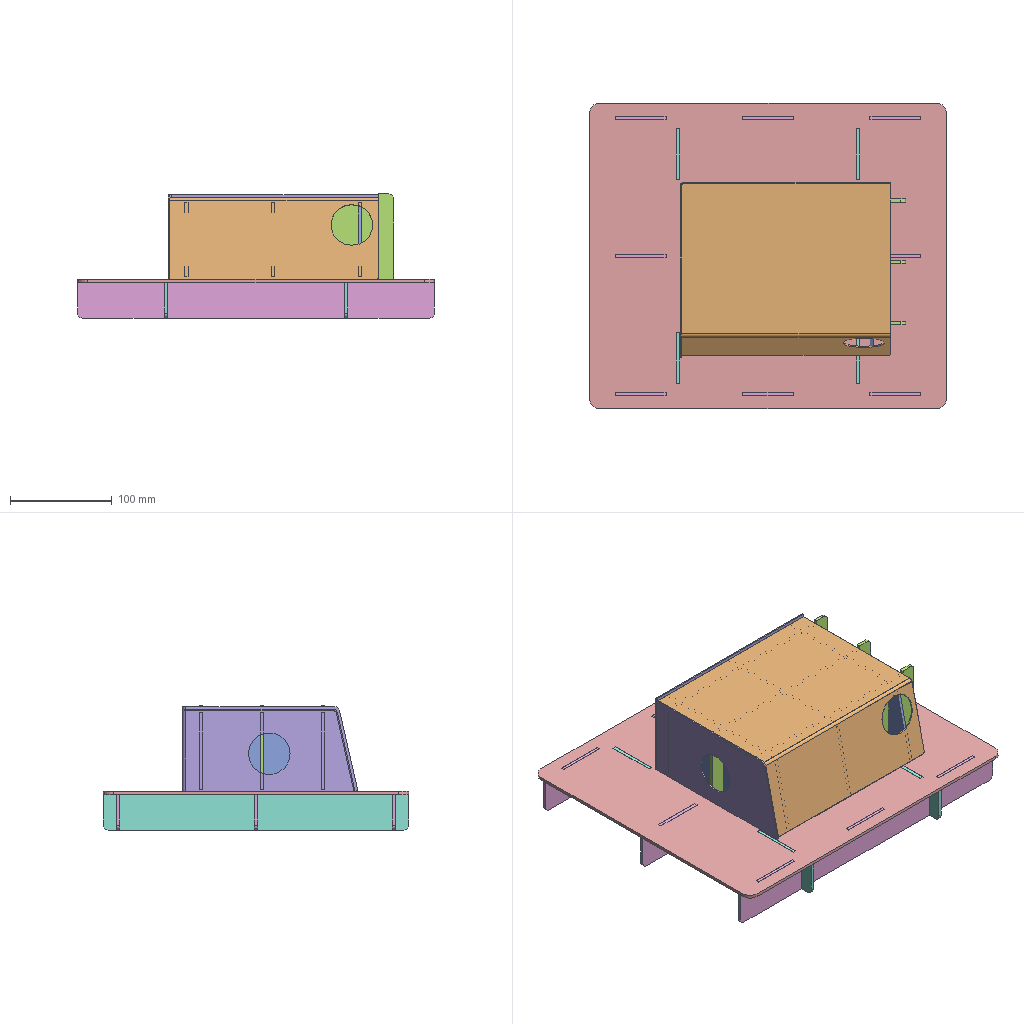Assembly | SolidWorks | 7 different items | 14 placed | box 350 x 300 x 122 mm
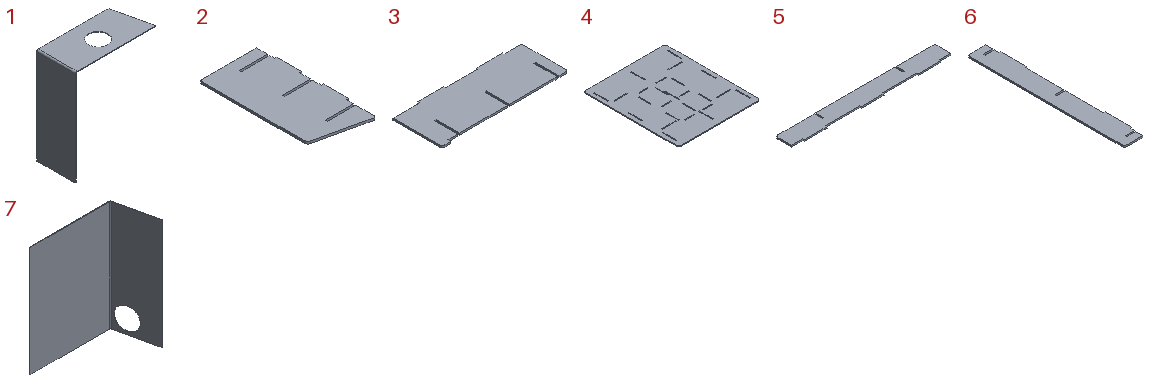Parts list (item | quantity | size | volume | features):
1 | x1 | 171.49 x 83 x 206 mm | 34881 mm3 | features Fillet 2, FlatPattern 1, ICE 1, SMBaseFlange 1, SheetMetal 1
2 | x3 | 81.8 x 166.27 x 3.2 mm | 39259 mm3 | features FlatPattern 1, SMBaseFlange 1, SheetMetal 1
3 | x3 | 219.8 x 86.8 x 3.2 mm | 55293 mm3 | features FlatPattern 1, SMBaseFlange 1, SheetMetal 1
4 | x1 | 300 x 350 x 3.2 mm | 324154 mm3 | features FlatPattern 1, SMBaseFlange 1, SheetMetal 1
5 | x3 | 350 x 38 x 3.2 mm | 40245 mm3 | features FlatPattern 1, SMBaseFlange 1, SheetMetal 1
6 | x2 | 38 x 300 x 3.2 mm | 33985 mm3 | features FlatPattern 1, SMBaseFlange 1, SheetMetal 1
7 | x1 | 168 x 80.263 x 204.8 mm | 55034 mm3 | features Fillet 1, FlatPattern 1, ICE 1, SMBaseFlange 1, SheetMetal 1
Mates (type | each side: item.copy, entity, surface, feature):
InPlace | 5.1 plane | assembly plane
InPlace | 6.1 plane | assembly plane
Coincident | 2.1 face plane Base-Flange1 | 7.1 face plane Base-Flange1
Coincident | 2.2 face plane Base-Flange1 | 7.1 face plane Base-Flange1
Coincident | 3.1 face plane Base-Flange1 | 7.1 face plane Base-Flange1
Coincident | 2.2 face plane Base-Flange1 | 1.1 face plane Base-Flange1
Coincident | 3.2 face plane Base-Flange1 | 1.1 face plane Base-Flange1
Coincident | 4.1 face plane Base-Flange1 | 1.1 face plane Base-Flange1